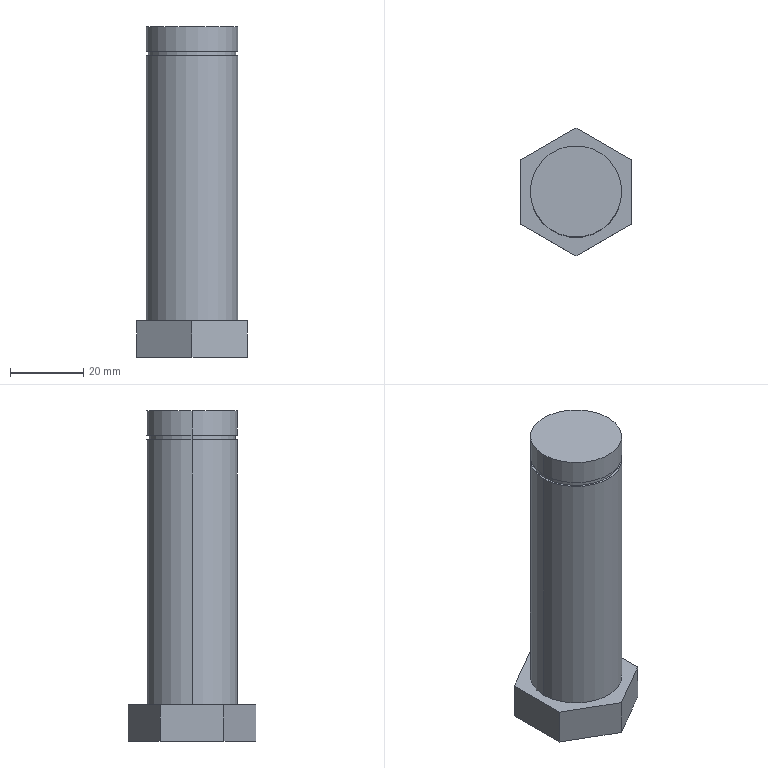Part | STEP file | 1 solid | 17 faces | box 30.311 x 35 x 90.5 mm | volume 47417 mm3 | plane 11 | cylinder 6 | commonest cylinder face diameters 25 x4 23.9 x2
STEP:
#1=CARTESIAN_POINT('',(0.,0.,0.));
#2=DIRECTION('',(0.,0.,1.));
#3=DIRECTION('',(1.,0.,0.));
#4=AXIS2_PLACEMENT_3D('',#1,#2,#3);
#5=CARTESIAN_POINT('',(-15.155,8.75,0.));
#6=VERTEX_POINT('',#5);
#7=CARTESIAN_POINT('',(0.,17.5,0.));
#8=VERTEX_POINT('',#7);
#9=CARTESIAN_POINT('',(-15.155,8.75,0.));
#10=DIRECTION('',(0.866,0.5,0.));
#11=VECTOR('',#10,1.);
#12=LINE('',#9,#11);
#13=CARTESIAN_POINT('',(0.,0.,0.));
#14=DIRECTION('',(0.,0.,1.));
#15=DIRECTION('',(1.,0.,0.));
#16=AXIS2_PLACEMENT_3D('',#13,#14,#15);
#17=PLANE('',#16);
#18=CARTESIAN_POINT('',(-15.155,8.75));
#19=DIRECTION('',(0.866,0.5));
#20=VECTOR('',#19,1.);
#21=LINE('',#18,#20);
#22=(GEOMETRIC_REPRESENTATION_CONTEXT(2)PARAMETRIC_REPRESENTATION_CONTEXT()REPRESENTATION_CONTEXT('',''));
#23=DEFINITIONAL_REPRESENTATION('',(#21),#22);
#24=PCURVE('',#17,#23);
#25=CARTESIAN_POINT('',(-15.155,8.75,10.));
#26=DIRECTION('',(-0.5,0.866,0.));
#27=DIRECTION('',(0.,0.,1.));
#28=AXIS2_PLACEMENT_3D('',#25,#26,#27);
#29=PLANE('',#28);
#30=CARTESIAN_POINT('',(-10.,0.));
#31=DIRECTION('',(0.,1.));
#32=VECTOR('',#31,1.);
#33=LINE('',#30,#32);
#34=(GEOMETRIC_REPRESENTATION_CONTEXT(2)PARAMETRIC_REPRESENTATION_CONTEXT()REPRESENTATION_CONTEXT('',''));
#35=DEFINITIONAL_REPRESENTATION('',(#33),#34);
#36=PCURVE('',#29,#35);
#37=SURFACE_CURVE('',#12,(#24,#36),.PCURVE_S1.);
#38=EDGE_CURVE('',#6,#8,#37,.T.);
#39=ORIENTED_EDGE('',*,*,#38,.T.);
#40=CARTESIAN_POINT('',(15.155,8.75,0.));
#41=VERTEX_POINT('',#40);
#42=CARTESIAN_POINT('',(0.,17.5,0.));
#43=DIRECTION('',(0.866,-0.5,0.));
#44=VECTOR('',#43,1.);
#45=LINE('',#42,#44);
#46=CARTESIAN_POINT('',(0.,17.5));
#47=DIRECTION('',(0.866,-0.5));
#48=VECTOR('',#47,1.);
#49=LINE('',#46,#48);
#50=(GEOMETRIC_REPRESENTATION_CONTEXT(2)PARAMETRIC_REPRESENTATION_CONTEXT()REPRESENTATION_CONTEXT('',''));
#51=DEFINITIONAL_REPRESENTATION('',(#49),#50);
#52=PCURVE('',#17,#51);
#53=CARTESIAN_POINT('',(0.,17.5,10.));
#54=DIRECTION('',(0.5,0.866,0.));
#55=DIRECTION('',(0.,0.,-1.));
#56=AXIS2_PLACEMENT_3D('',#53,#54,#55);
#57=PLANE('',#56);
#58=CARTESIAN_POINT('',(10.,0.));
#59=DIRECTION('',(0.,-1.));
#60=VECTOR('',#59,1.);
#61=LINE('',#58,#60);
#62=(GEOMETRIC_REPRESENTATION_CONTEXT(2)PARAMETRIC_REPRESENTATION_CONTEXT()REPRESENTATION_CONTEXT('',''));
#63=DEFINITIONAL_REPRESENTATION('',(#61),#62);
#64=PCURVE('',#57,#63);
#65=SURFACE_CURVE('',#45,(#52,#64),.PCURVE_S1.);
#66=EDGE_CURVE('',#8,#41,#65,.T.);
#67=ORIENTED_EDGE('',*,*,#66,.T.);
#68=CARTESIAN_POINT('',(15.155,-8.75,0.));
#69=VERTEX_POINT('',#68);
#70=CARTESIAN_POINT('',(15.155,8.75,0.));
#71=DIRECTION('',(0.,-1.,0.));
#72=VECTOR('',#71,1.);
#73=LINE('',#70,#72);
#74=CARTESIAN_POINT('',(15.155,8.75));
#75=DIRECTION('',(0.,-1.));
#76=VECTOR('',#75,1.);
#77=LINE('',#74,#76);
#78=(GEOMETRIC_REPRESENTATION_CONTEXT(2)PARAMETRIC_REPRESENTATION_CONTEXT()REPRESENTATION_CONTEXT('',''));
#79=DEFINITIONAL_REPRESENTATION('',(#77),#78);
#80=PCURVE('',#17,#79);
#81=CARTESIAN_POINT('',(15.155,8.75,10.));
#82=DIRECTION('',(1.,0.,0.));
#83=DIRECTION('',(0.,-1.,0.));
#84=AXIS2_PLACEMENT_3D('',#81,#82,#83);
#85=PLANE('',#84);
#86=CARTESIAN_POINT('',(0.,10.));
#87=DIRECTION('',(1.,0.));
#88=VECTOR('',#87,1.);
#89=LINE('',#86,#88);
#90=(GEOMETRIC_REPRESENTATION_CONTEXT(2)PARAMETRIC_REPRESENTATION_CONTEXT()REPRESENTATION_CONTEXT('',''));
#91=DEFINITIONAL_REPRESENTATION('',(#89),#90);
#92=PCURVE('',#85,#91);
#93=SURFACE_CURVE('',#73,(#80,#92),.PCURVE_S1.);
#94=EDGE_CURVE('',#41,#69,#93,.T.);
#95=ORIENTED_EDGE('',*,*,#94,.T.);
#96=CARTESIAN_POINT('',(0.,-17.5,0.));
#97=VERTEX_POINT('',#96);
#98=CARTESIAN_POINT('',(15.155,-8.75,0.));
#99=DIRECTION('',(-0.866,-0.5,0.));
#100=VECTOR('',#99,1.);
#101=LINE('',#98,#100);
#102=CARTESIAN_POINT('',(15.155,-8.75));
#103=DIRECTION('',(-0.866,-0.5));
#104=VECTOR('',#103,1.);
#105=LINE('',#102,#104);
#106=(GEOMETRIC_REPRESENTATION_CONTEXT(2)PARAMETRIC_REPRESENTATION_CONTEXT()REPRESENTATION_CONTEXT('',''));
#107=DEFINITIONAL_REPRESENTATION('',(#105),#106);
#108=PCURVE('',#17,#107);
#109=CARTESIAN_POINT('',(15.155,-8.75,10.));
#110=DIRECTION('',(0.5,-0.866,0.));
#111=DIRECTION('',(0.,0.,-1.));
#112=AXIS2_PLACEMENT_3D('',#109,#110,#111);
#113=PLANE('',#112);
#114=CARTESIAN_POINT('',(10.,0.));
#115=DIRECTION('',(0.,-1.));
#116=VECTOR('',#115,1.);
#117=LINE('',#114,#116);
#118=(GEOMETRIC_REPRESENTATION_CONTEXT(2)PARAMETRIC_REPRESENTATION_CONTEXT()REPRESENTATION_CONTEXT('',''));
#119=DEFINITIONAL_REPRESENTATION('',(#117),#118);
#120=PCURVE('',#113,#119);
#121=SURFACE_CURVE('',#101,(#108,#120),.PCURVE_S1.);
#122=EDGE_CURVE('',#69,#97,#121,.T.);
#123=ORIENTED_EDGE('',*,*,#122,.T.);
#124=CARTESIAN_POINT('',(-15.155,-8.75,0.));
#125=VERTEX_POINT('',#124);
#126=CARTESIAN_POINT('',(0.,-17.5,0.));
#127=DIRECTION('',(-0.866,0.5,0.));
#128=VECTOR('',#127,1.);
#129=LINE('',#126,#128);
#130=CARTESIAN_POINT('',(0.,-17.5));
#131=DIRECTION('',(-0.866,0.5));
#132=VECTOR('',#131,1.);
#133=LINE('',#130,#132);
#134=(GEOMETRIC_REPRESENTATION_CONTEXT(2)PARAMETRIC_REPRESENTATION_CONTEXT()REPRESENTATION_CONTEXT('',''));
#135=DEFINITIONAL_REPRESENTATION('',(#133),#134);
#136=PCURVE('',#17,#135);
#137=CARTESIAN_POINT('',(0.,-17.5,10.));
#138=DIRECTION('',(-0.5,-0.866,0.));
#139=DIRECTION('',(-0.866,0.5,0.));
#140=AXIS2_PLACEMENT_3D('',#137,#138,#139);
#141=PLANE('',#140);
#142=CARTESIAN_POINT('',(0.,10.));
#143=DIRECTION('',(1.,0.));
#144=VECTOR('',#143,1.);
#145=LINE('',#142,#144);
#146=(GEOMETRIC_REPRESENTATION_CONTEXT(2)PARAMETRIC_REPRESENTATION_CONTEXT()REPRESENTATION_CONTEXT('',''));
#147=DEFINITIONAL_REPRESENTATION('',(#145),#146);
#148=PCURVE('',#141,#147);
#149=SURFACE_CURVE('',#129,(#136,#148),.PCURVE_S1.);
#150=EDGE_CURVE('',#97,#125,#149,.T.);
#151=ORIENTED_EDGE('',*,*,#150,.T.);
#152=CARTESIAN_POINT('',(-15.155,-8.75,0.));
#153=DIRECTION('',(0.,1.,0.));
#154=VECTOR('',#153,1.);
#155=LINE('',#152,#154);
#156=CARTESIAN_POINT('',(-15.155,-8.75));
#157=DIRECTION('',(0.,1.));
#158=VECTOR('',#157,1.);
#159=LINE('',#156,#158);
#160=(GEOMETRIC_REPRESENTATION_CONTEXT(2)PARAMETRIC_REPRESENTATION_CONTEXT()REPRESENTATION_CONTEXT('',''));
#161=DEFINITIONAL_REPRESENTATION('',(#159),#160);
#162=PCURVE('',#17,#161);
#163=CARTESIAN_POINT('',(-15.155,-8.75,10.));
#164=DIRECTION('',(-1.,0.,0.));
#165=DIRECTION('',(0.,0.,1.));
#166=AXIS2_PLACEMENT_3D('',#163,#164,#165);
#167=PLANE('',#166);
#168=CARTESIAN_POINT('',(-10.,0.));
#169=DIRECTION('',(0.,1.));
#170=VECTOR('',#169,1.);
#171=LINE('',#168,#170);
#172=(GEOMETRIC_REPRESENTATION_CONTEXT(2)PARAMETRIC_REPRESENTATION_CONTEXT()REPRESENTATION_CONTEXT('',''));
#173=DEFINITIONAL_REPRESENTATION('',(#171),#172);
#174=PCURVE('',#167,#173);
#175=SURFACE_CURVE('',#155,(#162,#174),.PCURVE_S1.);
#176=EDGE_CURVE('',#125,#6,#175,.T.);
#177=ORIENTED_EDGE('',*,*,#176,.T.);
#178=EDGE_LOOP('',(#39,#67,#95,#123,#151,#177));
#179=FACE_BOUND('',#178,.T.);
#180=ADVANCED_FACE('',(#179),#17,.F.);
#181=ORIENTED_EDGE('',*,*,#66,.F.);
#182=CARTESIAN_POINT('',(0.,17.5,10.));
#183=VERTEX_POINT('',#182);
#184=CARTESIAN_POINT('',(0.,17.5,10.));
#185=DIRECTION('',(0.,0.,-1.));
#186=VECTOR('',#185,1.);
#187=LINE('',#184,#186);
#188=CARTESIAN_POINT('',(0.,0.));
#189=DIRECTION('',(1.,0.));
#190=VECTOR('',#189,1.);
#191=LINE('',#188,#190);
#192=(GEOMETRIC_REPRESENTATION_CONTEXT(2)PARAMETRIC_REPRESENTATION_CONTEXT()REPRESENTATION_CONTEXT('',''));
#193=DEFINITIONAL_REPRESENTATION('',(#191),#192);
#194=PCURVE('',#57,#193);
#195=CARTESIAN_POINT('',(0.,17.5));
#196=DIRECTION('',(-1.,0.));
#197=VECTOR('',#196,1.);
#198=LINE('',#195,#197);
#199=(GEOMETRIC_REPRESENTATION_CONTEXT(2)PARAMETRIC_REPRESENTATION_CONTEXT()REPRESENTATION_CONTEXT('',''));
#200=DEFINITIONAL_REPRESENTATION('',(#198),#199);
#201=PCURVE('',#29,#200);
#202=SURFACE_CURVE('',#187,(#194,#201),.PCURVE_S1.);
#203=EDGE_CURVE('',#183,#8,#202,.T.);
#204=ORIENTED_EDGE('',*,*,#203,.F.);
#205=CARTESIAN_POINT('',(15.155,8.75,10.));
#206=VERTEX_POINT('',#205);
#207=CARTESIAN_POINT('',(0.,17.5,10.));
#208=DIRECTION('',(0.866,-0.5,0.));
#209=VECTOR('',#208,1.);
#210=LINE('',#207,#209);
#211=CARTESIAN_POINT('',(0.,0.));
#212=DIRECTION('',(0.,-1.));
#213=VECTOR('',#212,1.);
#214=LINE('',#211,#213);
#215=(GEOMETRIC_REPRESENTATION_CONTEXT(2)PARAMETRIC_REPRESENTATION_CONTEXT()REPRESENTATION_CONTEXT('',''));
#216=DEFINITIONAL_REPRESENTATION('',(#214),#215);
#217=PCURVE('',#57,#216);
#218=CARTESIAN_POINT('',(0.,0.,10.));
#219=DIRECTION('',(0.,0.,1.));
#220=DIRECTION('',(1.,0.,0.));
#221=AXIS2_PLACEMENT_3D('',#218,#219,#220);
#222=PLANE('',#221);
#223=CARTESIAN_POINT('',(0.,17.5));
#224=DIRECTION('',(0.866,-0.5));
#225=VECTOR('',#224,1.);
#226=LINE('',#223,#225);
#227=(GEOMETRIC_REPRESENTATION_CONTEXT(2)PARAMETRIC_REPRESENTATION_CONTEXT()REPRESENTATION_CONTEXT('',''));
#228=DEFINITIONAL_REPRESENTATION('',(#226),#227);
#229=PCURVE('',#222,#228);
#230=SURFACE_CURVE('',#210,(#217,#229),.PCURVE_S1.);
#231=EDGE_CURVE('',#183,#206,#230,.T.);
#232=ORIENTED_EDGE('',*,*,#231,.T.);
#233=CARTESIAN_POINT('',(15.155,8.75,10.));
#234=DIRECTION('',(0.,0.,-1.));
#235=VECTOR('',#234,1.);
#236=LINE('',#233,#235);
#237=CARTESIAN_POINT('',(0.,-17.5));
#238=DIRECTION('',(1.,0.));
#239=VECTOR('',#238,1.);
#240=LINE('',#237,#239);
#241=(GEOMETRIC_REPRESENTATION_CONTEXT(2)PARAMETRIC_REPRESENTATION_CONTEXT()REPRESENTATION_CONTEXT('',''));
#242=DEFINITIONAL_REPRESENTATION('',(#240),#241);
#243=PCURVE('',#57,#242);
#244=CARTESIAN_POINT('',(0.,0.));
#245=DIRECTION('',(0.,1.));
#246=VECTOR('',#245,1.);
#247=LINE('',#244,#246);
#248=(GEOMETRIC_REPRESENTATION_CONTEXT(2)PARAMETRIC_REPRESENTATION_CONTEXT()REPRESENTATION_CONTEXT('',''));
#249=DEFINITIONAL_REPRESENTATION('',(#247),#248);
#250=PCURVE('',#85,#249);
#251=SURFACE_CURVE('',#236,(#243,#250),.PCURVE_S1.);
#252=EDGE_CURVE('',#206,#41,#251,.T.);
#253=ORIENTED_EDGE('',*,*,#252,.T.);
#254=EDGE_LOOP('',(#181,#204,#232,#253));
#255=FACE_BOUND('',#254,.T.);
#256=ADVANCED_FACE('',(#255),#57,.T.);
#257=ORIENTED_EDGE('',*,*,#94,.F.);
#258=ORIENTED_EDGE('',*,*,#252,.F.);
#259=CARTESIAN_POINT('',(15.155,-8.75,10.));
#260=VERTEX_POINT('',#259);
#261=CARTESIAN_POINT('',(15.155,8.75,10.));
#262=DIRECTION('',(0.,-1.,0.));
#263=VECTOR('',#262,1.);
#264=LINE('',#261,#263);
#265=CARTESIAN_POINT('',(0.,0.));
#266=DIRECTION('',(1.,0.));
#267=VECTOR('',#266,1.);
#268=LINE('',#265,#267);
#269=(GEOMETRIC_REPRESENTATION_CONTEXT(2)PARAMETRIC_REPRESENTATION_CONTEXT()REPRESENTATION_CONTEXT('',''));
#270=DEFINITIONAL_REPRESENTATION('',(#268),#269);
#271=PCURVE('',#85,#270);
#272=CARTESIAN_POINT('',(15.155,8.75));
#273=DIRECTION('',(0.,-1.));
#274=VECTOR('',#273,1.);
#275=LINE('',#272,#274);
#276=(GEOMETRIC_REPRESENTATION_CONTEXT(2)PARAMETRIC_REPRESENTATION_CONTEXT()REPRESENTATION_CONTEXT('',''));
#277=DEFINITIONAL_REPRESENTATION('',(#275),#276);
#278=PCURVE('',#222,#277);
#279=SURFACE_CURVE('',#264,(#271,#278),.PCURVE_S1.);
#280=EDGE_CURVE('',#206,#260,#279,.T.);
#281=ORIENTED_EDGE('',*,*,#280,.T.);
#282=CARTESIAN_POINT('',(15.155,-8.75,10.));
#283=DIRECTION('',(0.,0.,-1.));
#284=VECTOR('',#283,1.);
#285=LINE('',#282,#284);
#286=CARTESIAN_POINT('',(17.5,0.));
#287=DIRECTION('',(0.,1.));
#288=VECTOR('',#287,1.);
#289=LINE('',#286,#288);
#290=(GEOMETRIC_REPRESENTATION_CONTEXT(2)PARAMETRIC_REPRESENTATION_CONTEXT()REPRESENTATION_CONTEXT('',''));
#291=DEFINITIONAL_REPRESENTATION('',(#289),#290);
#292=PCURVE('',#85,#291);
#293=CARTESIAN_POINT('',(0.,0.));
#294=DIRECTION('',(1.,0.));
#295=VECTOR('',#294,1.);
#296=LINE('',#293,#295);
#297=(GEOMETRIC_REPRESENTATION_CONTEXT(2)PARAMETRIC_REPRESENTATION_CONTEXT()REPRESENTATION_CONTEXT('',''));
#298=DEFINITIONAL_REPRESENTATION('',(#296),#297);
#299=PCURVE('',#113,#298);
#300=SURFACE_CURVE('',#285,(#292,#299),.PCURVE_S1.);
#301=EDGE_CURVE('',#260,#69,#300,.T.);
#302=ORIENTED_EDGE('',*,*,#301,.T.);
#303=EDGE_LOOP('',(#257,#258,#281,#302));
#304=FACE_BOUND('',#303,.T.);
#305=ADVANCED_FACE('',(#304),#85,.T.);
#306=ORIENTED_EDGE('',*,*,#122,.F.);
#307=ORIENTED_EDGE('',*,*,#301,.F.);
#308=CARTESIAN_POINT('',(0.,-17.5,10.));
#309=VERTEX_POINT('',#308);
#310=CARTESIAN_POINT('',(15.155,-8.75,10.));
#311=DIRECTION('',(-0.866,-0.5,0.));
#312=VECTOR('',#311,1.);
#313=LINE('',#310,#312);
#314=CARTESIAN_POINT('',(0.,0.));
#315=DIRECTION('',(0.,-1.));
#316=VECTOR('',#315,1.);
#317=LINE('',#314,#316);
#318=(GEOMETRIC_REPRESENTATION_CONTEXT(2)PARAMETRIC_REPRESENTATION_CONTEXT()REPRESENTATION_CONTEXT('',''));
#319=DEFINITIONAL_REPRESENTATION('',(#317),#318);
#320=PCURVE('',#113,#319);
#321=CARTESIAN_POINT('',(15.155,-8.75));
#322=DIRECTION('',(-0.866,-0.5));
#323=VECTOR('',#322,1.);
#324=LINE('',#321,#323);
#325=(GEOMETRIC_REPRESENTATION_CONTEXT(2)PARAMETRIC_REPRESENTATION_CONTEXT()REPRESENTATION_CONTEXT('',''));
#326=DEFINITIONAL_REPRESENTATION('',(#324),#325);
#327=PCURVE('',#222,#326);
#328=SURFACE_CURVE('',#313,(#320,#327),.PCURVE_S1.);
#329=EDGE_CURVE('',#260,#309,#328,.T.);
#330=ORIENTED_EDGE('',*,*,#329,.T.);
#331=CARTESIAN_POINT('',(0.,-17.5,10.));
#332=DIRECTION('',(0.,0.,-1.));
#333=VECTOR('',#332,1.);
#334=LINE('',#331,#333);
#335=CARTESIAN_POINT('',(0.,-17.5));
#336=DIRECTION('',(1.,0.));
#337=VECTOR('',#336,1.);
#338=LINE('',#335,#337);
#339=(GEOMETRIC_REPRESENTATION_CONTEXT(2)PARAMETRIC_REPRESENTATION_CONTEXT()REPRESENTATION_CONTEXT('',''));
#340=DEFINITIONAL_REPRESENTATION('',(#338),#339);
#341=PCURVE('',#113,#340);
#342=CARTESIAN_POINT('',(0.,0.));
#343=DIRECTION('',(0.,1.));
#344=VECTOR('',#343,1.);
#345=LINE('',#342,#344);
#346=(GEOMETRIC_REPRESENTATION_CONTEXT(2)PARAMETRIC_REPRESENTATION_CONTEXT()REPRESENTATION_CONTEXT('',''));
#347=DEFINITIONAL_REPRESENTATION('',(#345),#346);
#348=PCURVE('',#141,#347);
#349=SURFACE_CURVE('',#334,(#341,#348),.PCURVE_S1.);
#350=EDGE_CURVE('',#309,#97,#349,.T.);
#351=ORIENTED_EDGE('',*,*,#350,.T.);
#352=EDGE_LOOP('',(#306,#307,#330,#351));
#353=FACE_BOUND('',#352,.T.);
#354=ADVANCED_FACE('',(#353),#113,.T.);
#355=ORIENTED_EDGE('',*,*,#150,.F.);
#356=ORIENTED_EDGE('',*,*,#350,.F.);
#357=CARTESIAN_POINT('',(-15.155,-8.75,10.));
#358=VERTEX_POINT('',#357);
#359=CARTESIAN_POINT('',(0.,-17.5,10.));
#360=DIRECTION('',(-0.866,0.5,0.));
#361=VECTOR('',#360,1.);
#362=LINE('',#359,#361);
#363=CARTESIAN_POINT('',(0.,0.));
#364=DIRECTION('',(1.,0.));
#365=VECTOR('',#364,1.);
#366=LINE('',#363,#365);
#367=(GEOMETRIC_REPRESENTATION_CONTEXT(2)PARAMETRIC_REPRESENTATION_CONTEXT()REPRESENTATION_CONTEXT('',''));
#368=DEFINITIONAL_REPRESENTATION('',(#366),#367);
#369=PCURVE('',#141,#368);
#370=CARTESIAN_POINT('',(0.,-17.5));
#371=DIRECTION('',(-0.866,0.5));
#372=VECTOR('',#371,1.);
#373=LINE('',#370,#372);
#374=(GEOMETRIC_REPRESENTATION_CONTEXT(2)PARAMETRIC_REPRESENTATION_CONTEXT()REPRESENTATION_CONTEXT('',''));
#375=DEFINITIONAL_REPRESENTATION('',(#373),#374);
#376=PCURVE('',#222,#375);
#377=SURFACE_CURVE('',#362,(#369,#376),.PCURVE_S1.);
#378=EDGE_CURVE('',#309,#358,#377,.T.);
#379=ORIENTED_EDGE('',*,*,#378,.T.);
#380=CARTESIAN_POINT('',(-15.155,-8.75,10.));
#381=DIRECTION('',(0.,0.,-1.));
#382=VECTOR('',#381,1.);
#383=LINE('',#380,#382);
#384=CARTESIAN_POINT('',(17.5,0.));
#385=DIRECTION('',(0.,1.));
#386=VECTOR('',#385,1.);
#387=LINE('',#384,#386);
#388=(GEOMETRIC_REPRESENTATION_CONTEXT(2)PARAMETRIC_REPRESENTATION_CONTEXT()REPRESENTATION_CONTEXT('',''));
#389=DEFINITIONAL_REPRESENTATION('',(#387),#388);
#390=PCURVE('',#141,#389);
#391=CARTESIAN_POINT('',(0.,0.));
#392=DIRECTION('',(-1.,0.));
#393=VECTOR('',#392,1.);
#394=LINE('',#391,#393);
#395=(GEOMETRIC_REPRESENTATION_CONTEXT(2)PARAMETRIC_REPRESENTATION_CONTEXT()REPRESENTATION_CONTEXT('',''));
#396=DEFINITIONAL_REPRESENTATION('',(#394),#395);
#397=PCURVE('',#167,#396);
#398=SURFACE_CURVE('',#383,(#390,#397),.PCURVE_S1.);
#399=EDGE_CURVE('',#358,#125,#398,.T.);
#400=ORIENTED_EDGE('',*,*,#399,.T.);
#401=EDGE_LOOP('',(#355,#356,#379,#400));
#402=FACE_BOUND('',#401,.T.);
#403=ADVANCED_FACE('',(#402),#141,.T.);
#404=ORIENTED_EDGE('',*,*,#176,.F.);
#405=ORIENTED_EDGE('',*,*,#399,.F.);
#406=CARTESIAN_POINT('',(-15.155,8.75,10.));
#407=VERTEX_POINT('',#406);
#408=CARTESIAN_POINT('',(-15.155,-8.75,10.));
#409=DIRECTION('',(0.,1.,0.));
#410=VECTOR('',#409,1.);
#411=LINE('',#408,#410);
#412=CARTESIAN_POINT('',(0.,0.));
#413=DIRECTION('',(0.,1.));
#414=VECTOR('',#413,1.);
#415=LINE('',#412,#414);
#416=(GEOMETRIC_REPRESENTATION_CONTEXT(2)PARAMETRIC_REPRESENTATION_CONTEXT()REPRESENTATION_CONTEXT('',''));
#417=DEFINITIONAL_REPRESENTATION('',(#415),#416);
#418=PCURVE('',#167,#417);
#419=CARTESIAN_POINT('',(-15.155,-8.75));
#420=DIRECTION('',(0.,1.));
#421=VECTOR('',#420,1.);
#422=LINE('',#419,#421);
#423=(GEOMETRIC_REPRESENTATION_CONTEXT(2)PARAMETRIC_REPRESENTATION_CONTEXT()REPRESENTATION_CONTEXT('',''));
#424=DEFINITIONAL_REPRESENTATION('',(#422),#423);
#425=PCURVE('',#222,#424);
#426=SURFACE_CURVE('',#411,(#418,#425),.PCURVE_S1.);
#427=EDGE_CURVE('',#358,#407,#426,.T.);
#428=ORIENTED_EDGE('',*,*,#427,.T.);
#429=CARTESIAN_POINT('',(-15.155,8.75,10.));
#430=DIRECTION('',(0.,0.,-1.));
#431=VECTOR('',#430,1.);
#432=LINE('',#429,#431);
#433=CARTESIAN_POINT('',(0.,17.5));
#434=DIRECTION('',(-1.,0.));
#435=VECTOR('',#434,1.);
#436=LINE('',#433,#435);
#437=(GEOMETRIC_REPRESENTATION_CONTEXT(2)PARAMETRIC_REPRESENTATION_CONTEXT()REPRESENTATION_CONTEXT('',''));
#438=DEFINITIONAL_REPRESENTATION('',(#436),#437);
#439=PCURVE('',#167,#438);
#440=CARTESIAN_POINT('',(0.,0.));
#441=DIRECTION('',(-1.,0.));
#442=VECTOR('',#441,1.);
#443=LINE('',#440,#442);
#444=(GEOMETRIC_REPRESENTATION_CONTEXT(2)PARAMETRIC_REPRESENTATION_CONTEXT()REPRESENTATION_CONTEXT('',''));
#445=DEFINITIONAL_REPRESENTATION('',(#443),#444);
#446=PCURVE('',#29,#445);
#447=SURFACE_CURVE('',#432,(#439,#446),.PCURVE_S1.);
#448=EDGE_CURVE('',#407,#6,#447,.T.);
#449=ORIENTED_EDGE('',*,*,#448,.T.);
#450=EDGE_LOOP('',(#404,#405,#428,#449));
#451=FACE_BOUND('',#450,.T.);
#452=ADVANCED_FACE('',(#451),#167,.T.);
#453=ORIENTED_EDGE('',*,*,#38,.F.);
#454=ORIENTED_EDGE('',*,*,#448,.F.);
#455=CARTESIAN_POINT('',(-15.155,8.75,10.));
#456=DIRECTION('',(0.866,0.5,0.));
#457=VECTOR('',#456,1.);
#458=LINE('',#455,#457);
#459=CARTESIAN_POINT('',(0.,0.));
#460=DIRECTION('',(0.,1.));
#461=VECTOR('',#460,1.);
#462=LINE('',#459,#461);
#463=(GEOMETRIC_REPRESENTATION_CONTEXT(2)PARAMETRIC_REPRESENTATION_CONTEXT()REPRESENTATION_CONTEXT('',''));
#464=DEFINITIONAL_REPRESENTATION('',(#462),#463);
#465=PCURVE('',#29,#464);
#466=CARTESIAN_POINT('',(-15.155,8.75));
#467=DIRECTION('',(0.866,0.5));
#468=VECTOR('',#467,1.);
#469=LINE('',#466,#468);
#470=(GEOMETRIC_REPRESENTATION_CONTEXT(2)PARAMETRIC_REPRESENTATION_CONTEXT()REPRESENTATION_CONTEXT('',''));
#471=DEFINITIONAL_REPRESENTATION('',(#469),#470);
#472=PCURVE('',#222,#471);
#473=SURFACE_CURVE('',#458,(#465,#472),.PCURVE_S1.);
#474=EDGE_CURVE('',#407,#183,#473,.T.);
#475=ORIENTED_EDGE('',*,*,#474,.T.);
#476=ORIENTED_EDGE('',*,*,#203,.T.);
#477=EDGE_LOOP('',(#453,#454,#475,#476));
#478=FACE_BOUND('',#477,.T.);
#479=ADVANCED_FACE('',(#478),#29,.T.);
#480=CARTESIAN_POINT('',(12.5,0.,90.5));
#481=VERTEX_POINT('',#480);
#482=CARTESIAN_POINT('',(12.5,0.,83.8));
#483=VERTEX_POINT('',#482);
#484=CARTESIAN_POINT('',(12.5,0.,90.5));
#485=DIRECTION('',(0.,0.,-1.));
#486=VECTOR('',#485,1.);
#487=LINE('',#484,#486);
#488=CARTESIAN_POINT('',(0.,0.,90.5));
#489=DIRECTION('',(0.,0.,-1.));
#490=DIRECTION('',(-1.,0.,0.));
#491=AXIS2_PLACEMENT_3D('',#488,#489,#490);
#492=CYLINDRICAL_SURFACE('',#491,12.5);
#493=CARTESIAN_POINT('',(3.142,0.));
#494=DIRECTION('',(0.,1.));
#495=VECTOR('',#494,1.);
#496=LINE('',#493,#495);
#497=(GEOMETRIC_REPRESENTATION_CONTEXT(2)PARAMETRIC_REPRESENTATION_CONTEXT()REPRESENTATION_CONTEXT('',''));
#498=DEFINITIONAL_REPRESENTATION('',(#496),#497);
#499=PCURVE('',#492,#498);
#500=CARTESIAN_POINT('',(0.,0.,90.5));
#501=DIRECTION('',(0.,0.,-1.));
#502=DIRECTION('',(-1.,0.,0.));
#503=AXIS2_PLACEMENT_3D('',#500,#501,#502);
#504=CYLINDRICAL_SURFACE('',#503,12.5);
#505=CARTESIAN_POINT('',(3.142,0.));
#506=DIRECTION('',(0.,1.));
#507=VECTOR('',#506,1.);
#508=LINE('',#505,#507);
#509=(GEOMETRIC_REPRESENTATION_CONTEXT(2)PARAMETRIC_REPRESENTATION_CONTEXT()REPRESENTATION_CONTEXT('',''));
#510=DEFINITIONAL_REPRESENTATION('',(#508),#509);
#511=PCURVE('',#504,#510);
#512=SURFACE_CURVE('',#487,(#499,#511),.PCURVE_S1.);
#513=EDGE_CURVE('',#481,#483,#512,.T.);
#514=ORIENTED_EDGE('',*,*,#513,.F.);
#515=CARTESIAN_POINT('',(-12.5,0.,90.5));
#516=VERTEX_POINT('',#515);
#517=CARTESIAN_POINT('',(0.,0.,90.5));
#518=DIRECTION('',(0.,0.,1.));
#519=DIRECTION('',(1.,0.,0.));
#520=AXIS2_PLACEMENT_3D('',#517,#518,#519);
#521=CIRCLE('',#520,12.5);
#522=CARTESIAN_POINT('',(9.425,0.));
#523=DIRECTION('',(-1.,0.));
#524=VECTOR('',#523,1.);
#525=LINE('',#522,#524);
#526=(GEOMETRIC_REPRESENTATION_CONTEXT(2)PARAMETRIC_REPRESENTATION_CONTEXT()REPRESENTATION_CONTEXT('',''));
#527=DEFINITIONAL_REPRESENTATION('',(#525),#526);
#528=PCURVE('',#492,#527);
#529=CARTESIAN_POINT('',(0.,0.,90.5));
#530=DIRECTION('',(0.,0.,1.));
#531=DIRECTION('',(1.,0.,0.));
#532=AXIS2_PLACEMENT_3D('',#529,#530,#531);
#533=PLANE('',#532);
#534=CARTESIAN_POINT('',(0.,0.));
#535=DIRECTION('',(1.,0.));
#536=AXIS2_PLACEMENT_2D('',#534,#535);
#537=CIRCLE('',#536,12.5);
#538=(GEOMETRIC_REPRESENTATION_CONTEXT(2)PARAMETRIC_REPRESENTATION_CONTEXT()REPRESENTATION_CONTEXT('',''));
#539=DEFINITIONAL_REPRESENTATION('',(#537),#538);
#540=PCURVE('',#533,#539);
#541=SURFACE_CURVE('',#521,(#528,#540),.PCURVE_S1.);
#542=EDGE_CURVE('',#516,#481,#541,.T.);
#543=ORIENTED_EDGE('',*,*,#542,.F.);
#544=CARTESIAN_POINT('',(-12.5,0.,83.8));
#545=VERTEX_POINT('',#544);
#546=CARTESIAN_POINT('',(-12.5,0.,90.5));
#547=DIRECTION('',(0.,0.,-1.));
#548=VECTOR('',#547,1.);
#549=LINE('',#546,#548);
#550=CARTESIAN_POINT('',(6.283,0.));
#551=DIRECTION('',(0.,1.));
#552=VECTOR('',#551,1.);
#553=LINE('',#550,#552);
#554=(GEOMETRIC_REPRESENTATION_CONTEXT(2)PARAMETRIC_REPRESENTATION_CONTEXT()REPRESENTATION_CONTEXT('',''));
#555=DEFINITIONAL_REPRESENTATION('',(#553),#554);
#556=PCURVE('',#492,#555);
#557=CARTESIAN_POINT('',(0.,0.));
#558=DIRECTION('',(0.,1.));
#559=VECTOR('',#558,1.);
#560=LINE('',#557,#559);
#561=(GEOMETRIC_REPRESENTATION_CONTEXT(2)PARAMETRIC_REPRESENTATION_CONTEXT()REPRESENTATION_CONTEXT('',''));
#562=DEFINITIONAL_REPRESENTATION('',(#560),#561);
#563=PCURVE('',#504,#562);
#564=SURFACE_CURVE('',#549,(#556,#563),.PCURVE_S1.);
#565=EDGE_CURVE('',#516,#545,#564,.T.);
#566=ORIENTED_EDGE('',*,*,#565,.T.);
#567=CARTESIAN_POINT('',(0.,0.,83.8));
#568=DIRECTION('',(0.,0.,-1.));
#569=DIRECTION('',(-1.,0.,0.));
#570=AXIS2_PLACEMENT_3D('',#567,#568,#569);
#571=CIRCLE('',#570,12.5);
#572=CARTESIAN_POINT('',(0.,6.7));
#573=DIRECTION('',(1.,0.));
#574=VECTOR('',#573,1.);
#575=LINE('',#572,#574);
#576=(GEOMETRIC_REPRESENTATION_CONTEXT(2)PARAMETRIC_REPRESENTATION_CONTEXT()REPRESENTATION_CONTEXT('',''));
#577=DEFINITIONAL_REPRESENTATION('',(#575),#576);
#578=PCURVE('',#492,#577);
#579=CARTESIAN_POINT('',(0.,14.486,83.8));
#580=DIRECTION('',(0.,0.,-1.));
#581=DIRECTION('',(0.,-1.,0.));
#582=AXIS2_PLACEMENT_3D('',#579,#580,#581);
#583=PLANE('',#582);
#584=CARTESIAN_POINT('',(14.486,0.));
#585=DIRECTION('',(0.,1.));
#586=AXIS2_PLACEMENT_2D('',#584,#585);
#587=CIRCLE('',#586,12.5);
#588=(GEOMETRIC_REPRESENTATION_CONTEXT(2)PARAMETRIC_REPRESENTATION_CONTEXT()REPRESENTATION_CONTEXT('',''));
#589=DEFINITIONAL_REPRESENTATION('',(#587),#588);
#590=PCURVE('',#583,#589);
#591=SURFACE_CURVE('',#571,(#578,#590),.PCURVE_S1.);
#592=EDGE_CURVE('',#483,#545,#591,.T.);
#593=ORIENTED_EDGE('',*,*,#592,.F.);
#594=EDGE_LOOP('',(#514,#543,#566,#593));
#595=FACE_BOUND('',#594,.T.);
#596=ADVANCED_FACE('',(#595),#492,.T.);
#597=ORIENTED_EDGE('',*,*,#542,.T.);
#598=CARTESIAN_POINT('',(0.,0.,90.5));
#599=DIRECTION('',(0.,0.,1.));
#600=DIRECTION('',(1.,0.,0.));
#601=AXIS2_PLACEMENT_3D('',#598,#599,#600);
#602=CIRCLE('',#601,12.5);
#603=CARTESIAN_POINT('',(0.,0.));
#604=DIRECTION('',(1.,0.));
#605=AXIS2_PLACEMENT_2D('',#603,#604);
#606=CIRCLE('',#605,12.5);
#607=(GEOMETRIC_REPRESENTATION_CONTEXT(2)PARAMETRIC_REPRESENTATION_CONTEXT()REPRESENTATION_CONTEXT('',''));
#608=DEFINITIONAL_REPRESENTATION('',(#606),#607);
#609=PCURVE('',#533,#608);
#610=CARTESIAN_POINT('',(3.142,0.));
#611=DIRECTION('',(-1.,0.));
#612=VECTOR('',#611,1.);
#613=LINE('',#610,#612);
#614=(GEOMETRIC_REPRESENTATION_CONTEXT(2)PARAMETRIC_REPRESENTATION_CONTEXT()REPRESENTATION_CONTEXT('',''));
#615=DEFINITIONAL_REPRESENTATION('',(#613),#614);
#616=PCURVE('',#504,#615);
#617=SURFACE_CURVE('',#602,(#609,#616),.PCURVE_S1.);
#618=EDGE_CURVE('',#481,#516,#617,.T.);
#619=ORIENTED_EDGE('',*,*,#618,.T.);
#620=EDGE_LOOP('',(#597,#619));
#621=FACE_BOUND('',#620,.T.);
#622=ADVANCED_FACE('',(#621),#533,.T.);
#623=CARTESIAN_POINT('',(-11.95,0.,82.5));
#624=VERTEX_POINT('',#623);
#625=CARTESIAN_POINT('',(-11.95,0.,83.8));
#626=VERTEX_POINT('',#625);
#627=CARTESIAN_POINT('',(-11.95,0.,99.498));
#628=DIRECTION('',(0.,0.,1.));
#629=VECTOR('',#628,1.);
#630=LINE('',#627,#629);
#631=CARTESIAN_POINT('',(0.,0.,99.498));
#632=DIRECTION('',(0.,0.,1.));
#633=DIRECTION('',(1.,0.,0.));
#634=AXIS2_PLACEMENT_3D('',#631,#632,#633);
#635=CYLINDRICAL_SURFACE('',#634,11.95);
#636=CARTESIAN_POINT('',(3.142,0.));
#637=DIRECTION('',(0.,1.));
#638=VECTOR('',#637,1.);
#639=LINE('',#636,#638);
#640=(GEOMETRIC_REPRESENTATION_CONTEXT(2)PARAMETRIC_REPRESENTATION_CONTEXT()REPRESENTATION_CONTEXT('',''));
#641=DEFINITIONAL_REPRESENTATION('',(#639),#640);
#642=PCURVE('',#635,#641);
#643=CARTESIAN_POINT('',(0.,0.,99.498));
#644=DIRECTION('',(0.,0.,1.));
#645=DIRECTION('',(1.,0.,0.));
#646=AXIS2_PLACEMENT_3D('',#643,#644,#645);
#647=CYLINDRICAL_SURFACE('',#646,11.95);
#648=CARTESIAN_POINT('',(3.142,0.));
#649=DIRECTION('',(0.,1.));
#650=VECTOR('',#649,1.);
#651=LINE('',#648,#650);
#652=(GEOMETRIC_REPRESENTATION_CONTEXT(2)PARAMETRIC_REPRESENTATION_CONTEXT()REPRESENTATION_CONTEXT('',''));
#653=DEFINITIONAL_REPRESENTATION('',(#651),#652);
#654=PCURVE('',#647,#653);
#655=SURFACE_CURVE('',#630,(#642,#654),.PCURVE_S1.);
#656=EDGE_CURVE('',#624,#626,#655,.T.);
#657=ORIENTED_EDGE('',*,*,#656,.F.);
#658=CARTESIAN_POINT('',(11.95,0.,82.5));
#659=VERTEX_POINT('',#658);
#660=CARTESIAN_POINT('',(0.,0.,82.5));
#661=DIRECTION('',(0.,0.,1.));
#662=DIRECTION('',(1.,0.,0.));
#663=AXIS2_PLACEMENT_3D('',#660,#661,#662);
#664=CIRCLE('',#663,11.95);
#665=CARTESIAN_POINT('',(0.,-16.998));
#666=DIRECTION('',(1.,0.));
#667=VECTOR('',#666,1.);
#668=LINE('',#665,#667);
#669=(GEOMETRIC_REPRESENTATION_CONTEXT(2)PARAMETRIC_REPRESENTATION_CONTEXT()REPRESENTATION_CONTEXT('',''));
#670=DEFINITIONAL_REPRESENTATION('',(#668),#669);
#671=PCURVE('',#635,#670);
#672=CARTESIAN_POINT('',(0.,14.486,82.5));
#673=DIRECTION('',(0.,0.,1.));
#674=DIRECTION('',(1.,0.,0.));
#675=AXIS2_PLACEMENT_3D('',#672,#673,#674);
#676=PLANE('',#675);
#677=CARTESIAN_POINT('',(0.,-14.486));
#678=DIRECTION('',(1.,0.));
#679=AXIS2_PLACEMENT_2D('',#677,#678);
#680=CIRCLE('',#679,11.95);
#681=(GEOMETRIC_REPRESENTATION_CONTEXT(2)PARAMETRIC_REPRESENTATION_CONTEXT()REPRESENTATION_CONTEXT('',''));
#682=DEFINITIONAL_REPRESENTATION('',(#680),#681);
#683=PCURVE('',#676,#682);
#684=SURFACE_CURVE('',#664,(#671,#683),.PCURVE_S1.);
#685=EDGE_CURVE('',#624,#659,#684,.T.);
#686=ORIENTED_EDGE('',*,*,#685,.T.);
#687=CARTESIAN_POINT('',(11.95,0.,83.8));
#688=VERTEX_POINT('',#687);
#689=CARTESIAN_POINT('',(11.95,0.,99.498));
#690=DIRECTION('',(0.,0.,1.));
#691=VECTOR('',#690,1.);
#692=LINE('',#689,#691);
#693=CARTESIAN_POINT('',(6.283,0.));
#694=DIRECTION('',(0.,1.));
#695=VECTOR('',#694,1.);
#696=LINE('',#693,#695);
#697=(GEOMETRIC_REPRESENTATION_CONTEXT(2)PARAMETRIC_REPRESENTATION_CONTEXT()REPRESENTATION_CONTEXT('',''));
#698=DEFINITIONAL_REPRESENTATION('',(#696),#697);
#699=PCURVE('',#635,#698);
#700=CARTESIAN_POINT('',(0.,0.));
#701=DIRECTION('',(0.,1.));
#702=VECTOR('',#701,1.);
#703=LINE('',#700,#702);
#704=(GEOMETRIC_REPRESENTATION_CONTEXT(2)PARAMETRIC_REPRESENTATION_CONTEXT()REPRESENTATION_CONTEXT('',''));
#705=DEFINITIONAL_REPRESENTATION('',(#703),#704);
#706=PCURVE('',#647,#705);
#707=SURFACE_CURVE('',#692,(#699,#706),.PCURVE_S1.);
#708=EDGE_CURVE('',#659,#688,#707,.T.);
#709=ORIENTED_EDGE('',*,*,#708,.T.);
#710=CARTESIAN_POINT('',(0.,0.,83.8));
#711=DIRECTION('',(0.,0.,1.));
#712=DIRECTION('',(1.,0.,0.));
#713=AXIS2_PLACEMENT_3D('',#710,#711,#712);
#714=CIRCLE('',#713,11.95);
#715=CARTESIAN_POINT('',(0.,-15.698));
#716=DIRECTION('',(1.,0.));
#717=VECTOR('',#716,1.);
#718=LINE('',#715,#717);
#719=(GEOMETRIC_REPRESENTATION_CONTEXT(2)PARAMETRIC_REPRESENTATION_CONTEXT()REPRESENTATION_CONTEXT('',''));
#720=DEFINITIONAL_REPRESENTATION('',(#718),#719);
#721=PCURVE('',#635,#720);
#722=CARTESIAN_POINT('',(14.486,-11.95));
#723=CARTESIAN_POINT('',(-6.212,-11.95));
#724=CARTESIAN_POINT('',(4.137,5.975));
#725=CARTESIAN_POINT('',(14.486,23.9));
#726=CARTESIAN_POINT('',(24.835,5.975));
#727=CARTESIAN_POINT('',(35.184,-11.95));
#728=CARTESIAN_POINT('',(14.486,-11.95));
#729=(BOUNDED_CURVE()B_SPLINE_CURVE(2,(#722,#723,#724,#725,#726,#727,#728),.UNSPECIFIED.,.T.,.F.)B_SPLINE_CURVE_WITH_KNOTS((1,2,2,2,2,1),(-2.094,0.,2.094,4.189,6.283,8.378),.UNSPECIFIED.)CURVE()GEOMETRIC_REPRESENTATION_ITEM()RATIONAL_B_SPLINE_CURVE((1.,0.5,1.,0.5,1.,0.5,1.))REPRESENTATION_ITEM(''));
#730=(GEOMETRIC_REPRESENTATION_CONTEXT(2)PARAMETRIC_REPRESENTATION_CONTEXT()REPRESENTATION_CONTEXT('',''));
#731=DEFINITIONAL_REPRESENTATION('',(#729),#730);
#732=PCURVE('',#583,#731);
#733=SURFACE_CURVE('',#714,(#721,#732),.PCURVE_S1.);
#734=EDGE_CURVE('',#626,#688,#733,.T.);
#735=ORIENTED_EDGE('',*,*,#734,.F.);
#736=EDGE_LOOP('',(#657,#686,#709,#735));
#737=FACE_BOUND('',#736,.T.);
#738=ADVANCED_FACE('',(#737),#635,.T.);
#739=CARTESIAN_POINT('',(0.,0.,82.5));
#740=DIRECTION('',(0.,0.,1.));
#741=DIRECTION('',(1.,0.,0.));
#742=AXIS2_PLACEMENT_3D('',#739,#740,#741);
#743=CIRCLE('',#742,11.95);
#744=CARTESIAN_POINT('',(0.,-14.486));
#745=DIRECTION('',(1.,0.));
#746=AXIS2_PLACEMENT_2D('',#744,#745);
#747=CIRCLE('',#746,11.95);
#748=(GEOMETRIC_REPRESENTATION_CONTEXT(2)PARAMETRIC_REPRESENTATION_CONTEXT()REPRESENTATION_CONTEXT('',''));
#749=DEFINITIONAL_REPRESENTATION('',(#747),#748);
#750=PCURVE('',#676,#749);
#751=CARTESIAN_POINT('',(0.,-16.998));
#752=DIRECTION('',(1.,0.));
#753=VECTOR('',#752,1.);
#754=LINE('',#751,#753);
#755=(GEOMETRIC_REPRESENTATION_CONTEXT(2)PARAMETRIC_REPRESENTATION_CONTEXT()REPRESENTATION_CONTEXT('',''));
#756=DEFINITIONAL_REPRESENTATION('',(#754),#755);
#757=PCURVE('',#647,#756);
#758=SURFACE_CURVE('',#743,(#750,#757),.PCURVE_S1.);
#759=EDGE_CURVE('',#659,#624,#758,.T.);
#760=ORIENTED_EDGE('',*,*,#759,.F.);
#761=ORIENTED_EDGE('',*,*,#685,.F.);
#762=EDGE_LOOP('',(#760,#761));
#763=FACE_BOUND('',#762,.T.);
#764=CARTESIAN_POINT('',(-12.5,0.,82.5));
#765=VERTEX_POINT('',#764);
#766=CARTESIAN_POINT('',(12.5,0.,82.5));
#767=VERTEX_POINT('',#766);
#768=CARTESIAN_POINT('',(0.,0.,82.5));
#769=DIRECTION('',(0.,0.,1.));
#770=DIRECTION('',(1.,0.,0.));
#771=AXIS2_PLACEMENT_3D('',#768,#769,#770);
#772=CIRCLE('',#771,12.5);
#773=CARTESIAN_POINT('',(0.,-14.486));
#774=DIRECTION('',(1.,0.));
#775=AXIS2_PLACEMENT_2D('',#773,#774);
#776=CIRCLE('',#775,12.5);
#777=(GEOMETRIC_REPRESENTATION_CONTEXT(2)PARAMETRIC_REPRESENTATION_CONTEXT()REPRESENTATION_CONTEXT('',''));
#778=DEFINITIONAL_REPRESENTATION('',(#776),#777);
#779=PCURVE('',#676,#778);
#780=CARTESIAN_POINT('',(0.,0.,90.5));
#781=DIRECTION('',(0.,0.,-1.));
#782=DIRECTION('',(-1.,0.,0.));
#783=AXIS2_PLACEMENT_3D('',#780,#781,#782);
#784=CYLINDRICAL_SURFACE('',#783,12.5);
#785=CARTESIAN_POINT('',(9.425,8.));
#786=DIRECTION('',(-1.,0.));
#787=VECTOR('',#786,1.);
#788=LINE('',#785,#787);
#789=(GEOMETRIC_REPRESENTATION_CONTEXT(2)PARAMETRIC_REPRESENTATION_CONTEXT()REPRESENTATION_CONTEXT('',''));
#790=DEFINITIONAL_REPRESENTATION('',(#788),#789);
#791=PCURVE('',#784,#790);
#792=SURFACE_CURVE('',#772,(#779,#791),.PCURVE_S1.);
#793=EDGE_CURVE('',#765,#767,#792,.T.);
#794=ORIENTED_EDGE('',*,*,#793,.T.);
#795=CARTESIAN_POINT('',(0.,0.,82.5));
#796=DIRECTION('',(0.,0.,1.));
#797=DIRECTION('',(1.,0.,0.));
#798=AXIS2_PLACEMENT_3D('',#795,#796,#797);
#799=CIRCLE('',#798,12.5);
#800=CARTESIAN_POINT('',(0.,-14.486));
#801=DIRECTION('',(1.,0.));
#802=AXIS2_PLACEMENT_2D('',#800,#801);
#803=CIRCLE('',#802,12.5);
#804=(GEOMETRIC_REPRESENTATION_CONTEXT(2)PARAMETRIC_REPRESENTATION_CONTEXT()REPRESENTATION_CONTEXT('',''));
#805=DEFINITIONAL_REPRESENTATION('',(#803),#804);
#806=PCURVE('',#676,#805);
#807=CARTESIAN_POINT('',(0.,0.,90.5));
#808=DIRECTION('',(0.,0.,-1.));
#809=DIRECTION('',(-1.,0.,0.));
#810=AXIS2_PLACEMENT_3D('',#807,#808,#809);
#811=CYLINDRICAL_SURFACE('',#810,12.5);
#812=CARTESIAN_POINT('',(3.142,8.));
#813=DIRECTION('',(-1.,0.));
#814=VECTOR('',#813,1.);
#815=LINE('',#812,#814);
#816=(GEOMETRIC_REPRESENTATION_CONTEXT(2)PARAMETRIC_REPRESENTATION_CONTEXT()REPRESENTATION_CONTEXT('',''));
#817=DEFINITIONAL_REPRESENTATION('',(#815),#816);
#818=PCURVE('',#811,#817);
#819=SURFACE_CURVE('',#799,(#806,#818),.PCURVE_S1.);
#820=EDGE_CURVE('',#767,#765,#819,.T.);
#821=ORIENTED_EDGE('',*,*,#820,.T.);
#822=EDGE_LOOP('',(#794,#821));
#823=FACE_BOUND('',#822,.T.);
#824=ADVANCED_FACE('',(#763,#823),#676,.T.);
#825=CARTESIAN_POINT('',(0.,0.,83.8));
#826=DIRECTION('',(0.,0.,1.));
#827=DIRECTION('',(1.,0.,0.));
#828=AXIS2_PLACEMENT_3D('',#825,#826,#827);
#829=CIRCLE('',#828,11.95);
#830=CARTESIAN_POINT('',(14.486,-11.95));
#831=CARTESIAN_POINT('',(-6.212,-11.95));
#832=CARTESIAN_POINT('',(4.137,5.975));
#833=CARTESIAN_POINT('',(14.486,23.9));
#834=CARTESIAN_POINT('',(24.835,5.975));
#835=CARTESIAN_POINT('',(35.184,-11.95));
#836=CARTESIAN_POINT('',(14.486,-11.95));
#837=(BOUNDED_CURVE()B_SPLINE_CURVE(2,(#830,#831,#832,#833,#834,#835,#836),.UNSPECIFIED.,.T.,.F.)B_SPLINE_CURVE_WITH_KNOTS((1,2,2,2,2,1),(-2.094,0.,2.094,4.189,6.283,8.378),.UNSPECIFIED.)CURVE()GEOMETRIC_REPRESENTATION_ITEM()RATIONAL_B_SPLINE_CURVE((1.,0.5,1.,0.5,1.,0.5,1.))REPRESENTATION_ITEM(''));
#838=(GEOMETRIC_REPRESENTATION_CONTEXT(2)PARAMETRIC_REPRESENTATION_CONTEXT()REPRESENTATION_CONTEXT('',''));
#839=DEFINITIONAL_REPRESENTATION('',(#837),#838);
#840=PCURVE('',#583,#839);
#841=CARTESIAN_POINT('',(0.,-15.698));
#842=DIRECTION('',(1.,0.));
#843=VECTOR('',#842,1.);
#844=LINE('',#841,#843);
#845=(GEOMETRIC_REPRESENTATION_CONTEXT(2)PARAMETRIC_REPRESENTATION_CONTEXT()REPRESENTATION_CONTEXT('',''));
#846=DEFINITIONAL_REPRESENTATION('',(#844),#845);
#847=PCURVE('',#647,#846);
#848=SURFACE_CURVE('',#829,(#840,#847),.PCURVE_S1.);
#849=EDGE_CURVE('',#688,#626,#848,.T.);
#850=ORIENTED_EDGE('',*,*,#849,.T.);
#851=ORIENTED_EDGE('',*,*,#734,.T.);
#852=EDGE_LOOP('',(#850,#851));
#853=FACE_BOUND('',#852,.T.);
#854=CARTESIAN_POINT('',(0.,0.,83.8));
#855=DIRECTION('',(0.,0.,-1.));
#856=DIRECTION('',(-1.,0.,0.));
#857=AXIS2_PLACEMENT_3D('',#854,#855,#856);
#858=CIRCLE('',#857,12.5);
#859=CARTESIAN_POINT('',(14.486,0.));
#860=DIRECTION('',(0.,1.));
#861=AXIS2_PLACEMENT_2D('',#859,#860);
#862=CIRCLE('',#861,12.5);
#863=(GEOMETRIC_REPRESENTATION_CONTEXT(2)PARAMETRIC_REPRESENTATION_CONTEXT()REPRESENTATION_CONTEXT('',''));
#864=DEFINITIONAL_REPRESENTATION('',(#862),#863);
#865=PCURVE('',#583,#864);
#866=CARTESIAN_POINT('',(0.,6.7));
#867=DIRECTION('',(1.,0.));
#868=VECTOR('',#867,1.);
#869=LINE('',#866,#868);
#870=(GEOMETRIC_REPRESENTATION_CONTEXT(2)PARAMETRIC_REPRESENTATION_CONTEXT()REPRESENTATION_CONTEXT('',''));
#871=DEFINITIONAL_REPRESENTATION('',(#869),#870);
#872=PCURVE('',#504,#871);
#873=SURFACE_CURVE('',#858,(#865,#872),.PCURVE_S1.);
#874=EDGE_CURVE('',#545,#483,#873,.T.);
#875=ORIENTED_EDGE('',*,*,#874,.T.);
#876=ORIENTED_EDGE('',*,*,#592,.T.);
#877=EDGE_LOOP('',(#875,#876));
#878=FACE_BOUND('',#877,.T.);
#879=ADVANCED_FACE('',(#853,#878),#583,.T.);
#880=CARTESIAN_POINT('',(12.5,0.,10.));
#881=VERTEX_POINT('',#880);
#882=CARTESIAN_POINT('',(12.5,0.,90.5));
#883=DIRECTION('',(0.,0.,-1.));
#884=VECTOR('',#883,1.);
#885=LINE('',#882,#884);
#886=CARTESIAN_POINT('',(3.142,0.));
#887=DIRECTION('',(0.,1.));
#888=VECTOR('',#887,1.);
#889=LINE('',#886,#888);
#890=(GEOMETRIC_REPRESENTATION_CONTEXT(2)PARAMETRIC_REPRESENTATION_CONTEXT()REPRESENTATION_CONTEXT('',''));
#891=DEFINITIONAL_REPRESENTATION('',(#889),#890);
#892=PCURVE('',#784,#891);
#893=CARTESIAN_POINT('',(3.142,0.));
#894=DIRECTION('',(0.,1.));
#895=VECTOR('',#894,1.);
#896=LINE('',#893,#895);
#897=(GEOMETRIC_REPRESENTATION_CONTEXT(2)PARAMETRIC_REPRESENTATION_CONTEXT()REPRESENTATION_CONTEXT('',''));
#898=DEFINITIONAL_REPRESENTATION('',(#896),#897);
#899=PCURVE('',#811,#898);
#900=SURFACE_CURVE('',#885,(#892,#899),.PCURVE_S1.);
#901=EDGE_CURVE('',#767,#881,#900,.T.);
#902=ORIENTED_EDGE('',*,*,#901,.F.);
#903=ORIENTED_EDGE('',*,*,#793,.F.);
#904=CARTESIAN_POINT('',(-12.5,0.,10.));
#905=VERTEX_POINT('',#904);
#906=CARTESIAN_POINT('',(-12.5,0.,90.5));
#907=DIRECTION('',(0.,0.,-1.));
#908=VECTOR('',#907,1.);
#909=LINE('',#906,#908);
#910=CARTESIAN_POINT('',(6.283,0.));
#911=DIRECTION('',(0.,1.));
#912=VECTOR('',#911,1.);
#913=LINE('',#910,#912);
#914=(GEOMETRIC_REPRESENTATION_CONTEXT(2)PARAMETRIC_REPRESENTATION_CONTEXT()REPRESENTATION_CONTEXT('',''));
#915=DEFINITIONAL_REPRESENTATION('',(#913),#914);
#916=PCURVE('',#784,#915);
#917=CARTESIAN_POINT('',(0.,0.));
#918=DIRECTION('',(0.,1.));
#919=VECTOR('',#918,1.);
#920=LINE('',#917,#919);
#921=(GEOMETRIC_REPRESENTATION_CONTEXT(2)PARAMETRIC_REPRESENTATION_CONTEXT()REPRESENTATION_CONTEXT('',''));
#922=DEFINITIONAL_REPRESENTATION('',(#920),#921);
#923=PCURVE('',#811,#922);
#924=SURFACE_CURVE('',#909,(#916,#923),.PCURVE_S1.);
#925=EDGE_CURVE('',#765,#905,#924,.T.);
#926=ORIENTED_EDGE('',*,*,#925,.T.);
#927=CARTESIAN_POINT('',(0.,0.,10.));
#928=DIRECTION('',(0.,0.,1.));
#929=DIRECTION('',(1.,0.,0.));
#930=AXIS2_PLACEMENT_3D('',#927,#928,#929);
#931=CIRCLE('',#930,12.5);
#932=CARTESIAN_POINT('',(9.425,80.5));
#933=DIRECTION('',(-1.,0.));
#934=VECTOR('',#933,1.);
#935=LINE('',#932,#934);
#936=(GEOMETRIC_REPRESENTATION_CONTEXT(2)PARAMETRIC_REPRESENTATION_CONTEXT()REPRESENTATION_CONTEXT('',''));
#937=DEFINITIONAL_REPRESENTATION('',(#935),#936);
#938=PCURVE('',#784,#937);
#939=CARTESIAN_POINT('',(0.,0.));
#940=DIRECTION('',(1.,0.));
#941=AXIS2_PLACEMENT_2D('',#939,#940);
#942=CIRCLE('',#941,12.5);
#943=(GEOMETRIC_REPRESENTATION_CONTEXT(2)PARAMETRIC_REPRESENTATION_CONTEXT()REPRESENTATION_CONTEXT('',''));
#944=DEFINITIONAL_REPRESENTATION('',(#942),#943);
#945=PCURVE('',#222,#944);
#946=SURFACE_CURVE('',#931,(#938,#945),.PCURVE_S1.);
#947=EDGE_CURVE('',#905,#881,#946,.T.);
#948=ORIENTED_EDGE('',*,*,#947,.T.);
#949=EDGE_LOOP('',(#902,#903,#926,#948));
#950=FACE_BOUND('',#949,.T.);
#951=ADVANCED_FACE('',(#950),#784,.T.);
#952=ORIENTED_EDGE('',*,*,#947,.F.);
#953=CARTESIAN_POINT('',(0.,0.,10.));
#954=DIRECTION('',(0.,0.,1.));
#955=DIRECTION('',(1.,0.,0.));
#956=AXIS2_PLACEMENT_3D('',#953,#954,#955);
#957=CIRCLE('',#956,12.5);
#958=CARTESIAN_POINT('',(0.,0.));
#959=DIRECTION('',(1.,0.));
#960=AXIS2_PLACEMENT_2D('',#958,#959);
#961=CIRCLE('',#960,12.5);
#962=(GEOMETRIC_REPRESENTATION_CONTEXT(2)PARAMETRIC_REPRESENTATION_CONTEXT()REPRESENTATION_CONTEXT('',''));
#963=DEFINITIONAL_REPRESENTATION('',(#961),#962);
#964=PCURVE('',#222,#963);
#965=CARTESIAN_POINT('',(3.142,80.5));
#966=DIRECTION('',(-1.,0.));
#967=VECTOR('',#966,1.);
#968=LINE('',#965,#967);
#969=(GEOMETRIC_REPRESENTATION_CONTEXT(2)PARAMETRIC_REPRESENTATION_CONTEXT()REPRESENTATION_CONTEXT('',''));
#970=DEFINITIONAL_REPRESENTATION('',(#968),#969);
#971=PCURVE('',#811,#970);
#972=SURFACE_CURVE('',#957,(#964,#971),.PCURVE_S1.);
#973=EDGE_CURVE('',#881,#905,#972,.T.);
#974=ORIENTED_EDGE('',*,*,#973,.F.);
#975=EDGE_LOOP('',(#952,#974));
#976=FACE_BOUND('',#975,.T.);
#977=ORIENTED_EDGE('',*,*,#231,.F.);
#978=ORIENTED_EDGE('',*,*,#474,.F.);
#979=ORIENTED_EDGE('',*,*,#427,.F.);
#980=ORIENTED_EDGE('',*,*,#378,.F.);
#981=ORIENTED_EDGE('',*,*,#329,.F.);
#982=ORIENTED_EDGE('',*,*,#280,.F.);
#983=EDGE_LOOP('',(#977,#978,#979,#980,#981,#982));
#984=FACE_BOUND('',#983,.T.);
#985=ADVANCED_FACE('',(#976,#984),#222,.T.);
#986=ORIENTED_EDGE('',*,*,#820,.F.);
#987=ORIENTED_EDGE('',*,*,#901,.T.);
#988=ORIENTED_EDGE('',*,*,#973,.T.);
#989=ORIENTED_EDGE('',*,*,#925,.F.);
#990=EDGE_LOOP('',(#986,#987,#988,#989));
#991=FACE_BOUND('',#990,.T.);
#992=ADVANCED_FACE('',(#991),#811,.T.);
#993=ORIENTED_EDGE('',*,*,#759,.T.);
#994=ORIENTED_EDGE('',*,*,#656,.T.);
#995=ORIENTED_EDGE('',*,*,#849,.F.);
#996=ORIENTED_EDGE('',*,*,#708,.F.);
#997=EDGE_LOOP('',(#993,#994,#995,#996));
#998=FACE_BOUND('',#997,.T.);
#999=ADVANCED_FACE('',(#998),#647,.T.);
#1000=ORIENTED_EDGE('',*,*,#618,.F.);
#1001=ORIENTED_EDGE('',*,*,#513,.T.);
#1002=ORIENTED_EDGE('',*,*,#874,.F.);
#1003=ORIENTED_EDGE('',*,*,#565,.F.);
#1004=EDGE_LOOP('',(#1000,#1001,#1002,#1003));
#1005=FACE_BOUND('',#1004,.T.);
#1006=ADVANCED_FACE('',(#1005),#504,.T.);
#1007=CLOSED_SHELL('',(#180,#256,#305,#354,#403,#452,#479,#596,#622,#738,#824,#879,#951,#985,#992,#999,#1006));
#1008=MANIFOLD_SOLID_BREP('',#1007);
#1009=(LENGTH_UNIT()NAMED_UNIT(*)SI_UNIT(.MILLI.,.METRE.));
#1010=UNCERTAINTY_MEASURE_WITH_UNIT(LENGTH_MEASURE(0.0000001),#1009,'','');
#1011=(NAMED_UNIT(*)PLANE_ANGLE_UNIT()SI_UNIT($,.RADIAN.));
#1012=(NAMED_UNIT(*)SI_UNIT($,.STERADIAN.)SOLID_ANGLE_UNIT());
#1013=(GEOMETRIC_REPRESENTATION_CONTEXT(3)GLOBAL_UNCERTAINTY_ASSIGNED_CONTEXT((#1010))GLOBAL_UNIT_ASSIGNED_CONTEXT((#1009,#1011,#1012))REPRESENTATION_CONTEXT('',''));
#1014=ADVANCED_BREP_SHAPE_REPRESENTATION('',(#4,#1008),#1013);